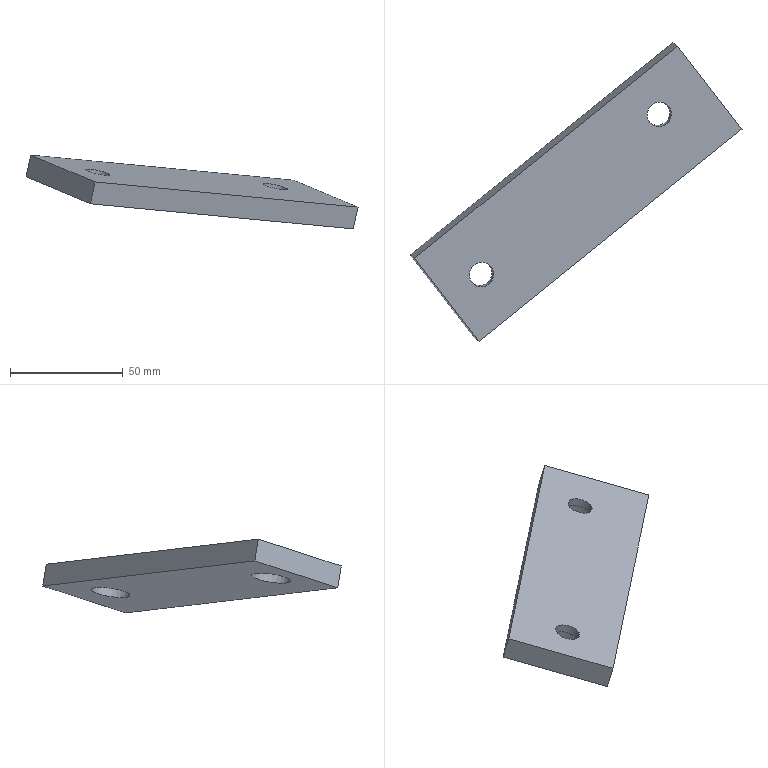Part | NX | features solid 2 | 1 solid | 12 faces | box 147.054 x 132.14 x 32.685 mm | volume 68266 mm3 | plane 8 | cylinder 4 | commonest cylinder face diameters 11 x2 17.5 x2
STEP:
#1=CARTESIAN_POINT('',(-157.138,684.094,54.963));
#2=VERTEX_POINT('',#1);
#3=CARTESIAN_POINT('',(-185.638,720.838,66.865));
#4=VERTEX_POINT('',#3);
#5=CARTESIAN_POINT('',(-185.638,720.838,66.865));
#6=DIRECTION('',(-0.5937,0.7655,0.248));
#7=VECTOR('',#6,1000.);
#8=LINE('',#5,#7);
#9=EDGE_CURVE('',#2,#4,#8,.T.);
#10=ORIENTED_EDGE('',*,*,#9,.T.);
#11=CARTESIAN_POINT('',(-187.758,722.323,57.206));
#12=VERTEX_POINT('',#11);
#13=CARTESIAN_POINT('',(-187.758,722.323,57.206));
#14=DIRECTION('',(0.212,-0.1485,0.9659));
#15=VECTOR('',#14,1000.);
#16=LINE('',#13,#15);
#17=EDGE_CURVE('',#12,#4,#16,.T.);
#18=ORIENTED_EDGE('',*,*,#17,.F.);
#19=CARTESIAN_POINT('',(-159.259,685.579,45.303));
#20=VERTEX_POINT('',#19);
#21=CARTESIAN_POINT('',(-187.758,722.323,57.206));
#22=DIRECTION('',(-0.5937,0.7655,0.248));
#23=VECTOR('',#22,1000.);
#24=LINE('',#21,#23);
#25=EDGE_CURVE('',#20,#12,#24,.T.);
#26=ORIENTED_EDGE('',*,*,#25,.F.);
#27=CARTESIAN_POINT('',(-159.259,685.579,45.303));
#28=DIRECTION('',(0.212,-0.1485,0.9659));
#29=VECTOR('',#28,1000.);
#30=LINE('',#27,#29);
#31=EDGE_CURVE('',#20,#2,#30,.T.);
#32=ORIENTED_EDGE('',*,*,#31,.T.);
#33=EDGE_LOOP('',(#10,#18,#26,#32));
#34=FACE_BOUND('',#33,.T.);
#35=CARTESIAN_POINT('',(-187.758,722.323,57.206));
#36=DIRECTION('',(0.7762,0.6261,-0.07415));
#37=DIRECTION('',(-0.6278,0.7784,0.));
#38=AXIS2_PLACEMENT_3D('',#35,#36,#37);
#39=PLANE('',#38);
#40=ADVANCED_FACE('',(#34),#39,.F.);
#41=CARTESIAN_POINT('',(-40.704,778.006,43.839));
#42=VERTEX_POINT('',#41);
#43=CARTESIAN_POINT('',(-40.704,778.006,43.839));
#44=DIRECTION('',(-0.7762,-0.6261,0.07415));
#45=VECTOR('',#44,1000.);
#46=LINE('',#43,#45);
#47=EDGE_CURVE('',#42,#2,#46,.T.);
#48=ORIENTED_EDGE('',*,*,#47,.T.);
#49=ORIENTED_EDGE('',*,*,#31,.F.);
#50=CARTESIAN_POINT('',(-42.824,779.49,34.18));
#51=VERTEX_POINT('',#50);
#52=CARTESIAN_POINT('',(-42.824,779.49,34.18));
#53=DIRECTION('',(-0.7762,-0.6261,0.07415));
#54=VECTOR('',#53,1000.);
#55=LINE('',#52,#54);
#56=EDGE_CURVE('',#51,#20,#55,.T.);
#57=ORIENTED_EDGE('',*,*,#56,.F.);
#58=CARTESIAN_POINT('',(-42.824,779.49,34.18));
#59=DIRECTION('',(0.212,-0.1485,0.9659));
#60=VECTOR('',#59,1000.);
#61=LINE('',#58,#60);
#62=EDGE_CURVE('',#51,#42,#61,.T.);
#63=ORIENTED_EDGE('',*,*,#62,.T.);
#64=EDGE_LOOP('',(#48,#49,#57,#63));
#65=FACE_BOUND('',#64,.T.);
#66=CARTESIAN_POINT('',(-42.824,779.49,34.18));
#67=DIRECTION('',(-0.5937,0.7655,0.248));
#68=DIRECTION('',(-0.7902,-0.6129,0.));
#69=AXIS2_PLACEMENT_3D('',#66,#67,#68);
#70=PLANE('',#69);
#71=ADVANCED_FACE('',(#65),#70,.F.);
#72=CARTESIAN_POINT('',(-69.203,814.75,55.742));
#73=VERTEX_POINT('',#72);
#74=CARTESIAN_POINT('',(-69.203,814.75,55.742));
#75=DIRECTION('',(-0.5937,0.7655,0.248));
#76=VECTOR('',#75,1000.);
#77=LINE('',#74,#76);
#78=EDGE_CURVE('',#42,#73,#77,.T.);
#79=ORIENTED_EDGE('',*,*,#78,.F.);
#80=ORIENTED_EDGE('',*,*,#62,.F.);
#81=CARTESIAN_POINT('',(-71.323,816.234,46.083));
#82=VERTEX_POINT('',#81);
#83=CARTESIAN_POINT('',(-71.323,816.234,46.083));
#84=DIRECTION('',(-0.5937,0.7655,0.248));
#85=VECTOR('',#84,1000.);
#86=LINE('',#83,#85);
#87=EDGE_CURVE('',#51,#82,#86,.T.);
#88=ORIENTED_EDGE('',*,*,#87,.T.);
#89=CARTESIAN_POINT('',(-71.323,816.234,46.083));
#90=DIRECTION('',(0.212,-0.1485,0.9659));
#91=VECTOR('',#90,1000.);
#92=LINE('',#89,#91);
#93=EDGE_CURVE('',#82,#73,#92,.T.);
#94=ORIENTED_EDGE('',*,*,#93,.T.);
#95=EDGE_LOOP('',(#79,#80,#88,#94));
#96=FACE_BOUND('',#95,.T.);
#97=CARTESIAN_POINT('',(-71.323,816.234,46.083));
#98=DIRECTION('',(0.7762,0.6261,-0.07415));
#99=DIRECTION('',(-0.6278,0.7784,0.));
#100=AXIS2_PLACEMENT_3D('',#97,#98,#99);
#101=PLANE('',#100);
#102=ADVANCED_FACE('',(#96),#101,.T.);
#103=CARTESIAN_POINT('',(-69.203,814.75,55.742));
#104=DIRECTION('',(-0.7762,-0.6261,0.07415));
#105=VECTOR('',#104,1000.);
#106=LINE('',#103,#105);
#107=EDGE_CURVE('',#73,#4,#106,.T.);
#108=ORIENTED_EDGE('',*,*,#107,.F.);
#109=ORIENTED_EDGE('',*,*,#93,.F.);
#110=CARTESIAN_POINT('',(-71.323,816.234,46.083));
#111=DIRECTION('',(-0.7762,-0.6261,0.07415));
#112=VECTOR('',#111,1000.);
#113=LINE('',#110,#112);
#114=EDGE_CURVE('',#82,#12,#113,.T.);
#115=ORIENTED_EDGE('',*,*,#114,.T.);
#116=ORIENTED_EDGE('',*,*,#17,.T.);
#117=EDGE_LOOP('',(#108,#109,#115,#116));
#118=FACE_BOUND('',#117,.T.);
#119=CARTESIAN_POINT('',(-71.323,816.234,46.083));
#120=DIRECTION('',(-0.5937,0.7655,0.248));
#121=DIRECTION('',(-0.7902,-0.6129,0.));
#122=AXIS2_PLACEMENT_3D('',#119,#120,#121);
#123=PLANE('',#122);
#124=ADVANCED_FACE('',(#118),#123,.T.);
#125=CARTESIAN_POINT('',(-149.62,715.081,47.722));
#126=VERTEX_POINT('',#125);
#127=CARTESIAN_POINT('',(-158.166,715.081,49.598));
#128=DIRECTION('',(0.212,-0.1485,0.9659));
#129=DIRECTION('',(0.9767,0.,-0.2144));
#130=AXIS2_PLACEMENT_3D('',#127,#128,#129);
#131=CIRCLE('',#130,8.75);
#132=EDGE_CURVE('',#126,#126,#131,.T.);
#133=ORIENTED_EDGE('',*,*,#132,.T.);
#134=EDGE_LOOP('',(#133));
#135=FACE_BOUND('',#134,.T.);
#136=CARTESIAN_POINT('',(-70.902,786.038,41.349));
#137=VERTEX_POINT('',#136);
#138=CARTESIAN_POINT('',(-79.448,786.038,43.225));
#139=DIRECTION('',(0.212,-0.1485,0.9659));
#140=DIRECTION('',(0.9767,0.,-0.2144));
#141=AXIS2_PLACEMENT_3D('',#138,#139,#140);
#142=CIRCLE('',#141,8.75);
#143=EDGE_CURVE('',#137,#137,#142,.T.);
#144=ORIENTED_EDGE('',*,*,#143,.T.);
#145=EDGE_LOOP('',(#144));
#146=FACE_BOUND('',#145,.T.);
#147=ORIENTED_EDGE('',*,*,#25,.T.);
#148=ORIENTED_EDGE('',*,*,#114,.F.);
#149=ORIENTED_EDGE('',*,*,#87,.F.);
#150=ORIENTED_EDGE('',*,*,#56,.T.);
#151=EDGE_LOOP('',(#147,#148,#149,#150));
#152=FACE_BOUND('',#151,.T.);
#153=CARTESIAN_POINT('',(-71.323,816.234,46.083));
#154=DIRECTION('',(0.212,-0.1485,0.9659));
#155=DIRECTION('',(-0.7762,-0.6261,0.07415));
#156=AXIS2_PLACEMENT_3D('',#153,#154,#155);
#157=PLANE('',#156);
#158=ADVANCED_FACE('',(#135,#146,#152),#157,.F.);
#159=CARTESIAN_POINT('',(-150.674,713.596,58.078));
#160=VERTEX_POINT('',#159);
#161=CARTESIAN_POINT('',(-156.046,713.596,59.257));
#162=DIRECTION('',(0.212,-0.1485,0.9659));
#163=DIRECTION('',(0.9767,0.,-0.2144));
#164=AXIS2_PLACEMENT_3D('',#161,#162,#163);
#165=CIRCLE('',#164,5.5);
#166=EDGE_CURVE('',#160,#160,#165,.T.);
#167=ORIENTED_EDGE('',*,*,#166,.F.);
#168=EDGE_LOOP('',(#167));
#169=FACE_BOUND('',#168,.T.);
#170=CARTESIAN_POINT('',(-71.956,784.553,51.705));
#171=VERTEX_POINT('',#170);
#172=CARTESIAN_POINT('',(-77.328,784.553,52.884));
#173=DIRECTION('',(0.212,-0.1485,0.9659));
#174=DIRECTION('',(0.9767,0.,-0.2144));
#175=AXIS2_PLACEMENT_3D('',#172,#173,#174);
#176=CIRCLE('',#175,5.5);
#177=EDGE_CURVE('',#171,#171,#176,.T.);
#178=ORIENTED_EDGE('',*,*,#177,.F.);
#179=EDGE_LOOP('',(#178));
#180=FACE_BOUND('',#179,.T.);
#181=ORIENTED_EDGE('',*,*,#9,.F.);
#182=ORIENTED_EDGE('',*,*,#47,.F.);
#183=ORIENTED_EDGE('',*,*,#78,.T.);
#184=ORIENTED_EDGE('',*,*,#107,.T.);
#185=EDGE_LOOP('',(#181,#182,#183,#184));
#186=FACE_BOUND('',#185,.T.);
#187=CARTESIAN_POINT('',(-69.203,814.75,55.742));
#188=DIRECTION('',(0.212,-0.1485,0.9659));
#189=DIRECTION('',(-0.7762,-0.6261,0.07415));
#190=AXIS2_PLACEMENT_3D('',#187,#188,#189);
#191=PLANE('',#190);
#192=ADVANCED_FACE('',(#169,#180,#186),#191,.T.);
#193=ORIENTED_EDGE('',*,*,#177,.T.);
#194=EDGE_LOOP('',(#193));
#195=FACE_BOUND('',#194,.T.);
#196=CARTESIAN_POINT('',(-72.74,785.103,48.131));
#197=VERTEX_POINT('',#196);
#198=CARTESIAN_POINT('',(-78.112,785.103,49.31));
#199=DIRECTION('',(0.212,-0.1485,0.9659));
#200=DIRECTION('',(0.9767,0.,-0.2144));
#201=AXIS2_PLACEMENT_3D('',#198,#199,#200);
#202=CIRCLE('',#201,5.5);
#203=EDGE_CURVE('',#197,#197,#202,.T.);
#204=ORIENTED_EDGE('',*,*,#203,.F.);
#205=EDGE_LOOP('',(#204));
#206=FACE_BOUND('',#205,.T.);
#207=CARTESIAN_POINT('',(-68.848,778.615,91.521));
#208=DIRECTION('',(0.212,-0.1485,0.9659));
#209=DIRECTION('',(0.9767,0.,-0.2144));
#210=AXIS2_PLACEMENT_3D('',#207,#208,#209);
#211=CYLINDRICAL_SURFACE('',#210,5.5);
#212=ADVANCED_FACE('',(#195,#206),#211,.F.);
#213=ORIENTED_EDGE('',*,*,#203,.T.);
#214=EDGE_LOOP('',(#213));
#215=FACE_BOUND('',#214,.T.);
#216=CARTESIAN_POINT('',(-69.566,785.103,47.435));
#217=VERTEX_POINT('',#216);
#218=CARTESIAN_POINT('',(-78.112,785.103,49.31));
#219=DIRECTION('',(0.212,-0.1485,0.9659));
#220=DIRECTION('',(0.9767,0.,-0.2144));
#221=AXIS2_PLACEMENT_3D('',#218,#219,#220);
#222=CIRCLE('',#221,8.75);
#223=EDGE_CURVE('',#217,#217,#222,.T.);
#224=ORIENTED_EDGE('',*,*,#223,.F.);
#225=EDGE_LOOP('',(#224));
#226=FACE_BOUND('',#225,.T.);
#227=CARTESIAN_POINT('',(-78.112,785.103,49.31));
#228=DIRECTION('',(0.212,-0.1485,0.9659));
#229=DIRECTION('',(0.9767,0.,-0.2144));
#230=AXIS2_PLACEMENT_3D('',#227,#228,#229);
#231=PLANE('',#230);
#232=ADVANCED_FACE('',(#215,#226),#231,.F.);
#233=ORIENTED_EDGE('',*,*,#223,.T.);
#234=EDGE_LOOP('',(#233));
#235=FACE_BOUND('',#234,.T.);
#236=ORIENTED_EDGE('',*,*,#143,.F.);
#237=EDGE_LOOP('',(#236));
#238=FACE_BOUND('',#237,.T.);
#239=CARTESIAN_POINT('',(-79.448,786.038,43.225));
#240=DIRECTION('',(0.212,-0.1485,0.9659));
#241=DIRECTION('',(0.9767,0.,-0.2144));
#242=AXIS2_PLACEMENT_3D('',#239,#240,#241);
#243=CYLINDRICAL_SURFACE('',#242,8.75);
#244=ADVANCED_FACE('',(#235,#238),#243,.F.);
#245=ORIENTED_EDGE('',*,*,#166,.T.);
#246=EDGE_LOOP('',(#245));
#247=FACE_BOUND('',#246,.T.);
#248=CARTESIAN_POINT('',(-151.458,714.146,54.504));
#249=VERTEX_POINT('',#248);
#250=CARTESIAN_POINT('',(-156.83,714.146,55.683));
#251=DIRECTION('',(0.212,-0.1485,0.9659));
#252=DIRECTION('',(0.9767,0.,-0.2144));
#253=AXIS2_PLACEMENT_3D('',#250,#251,#252);
#254=CIRCLE('',#253,5.5);
#255=EDGE_CURVE('',#249,#249,#254,.T.);
#256=ORIENTED_EDGE('',*,*,#255,.F.);
#257=EDGE_LOOP('',(#256));
#258=FACE_BOUND('',#257,.T.);
#259=CARTESIAN_POINT('',(-147.565,707.658,97.894));
#260=DIRECTION('',(0.212,-0.1485,0.9659));
#261=DIRECTION('',(0.9767,0.,-0.2144));
#262=AXIS2_PLACEMENT_3D('',#259,#260,#261);
#263=CYLINDRICAL_SURFACE('',#262,5.5);
#264=ADVANCED_FACE('',(#247,#258),#263,.F.);
#265=ORIENTED_EDGE('',*,*,#255,.T.);
#266=EDGE_LOOP('',(#265));
#267=FACE_BOUND('',#266,.T.);
#268=CARTESIAN_POINT('',(-148.284,714.146,53.807));
#269=VERTEX_POINT('',#268);
#270=CARTESIAN_POINT('',(-156.83,714.146,55.683));
#271=DIRECTION('',(0.212,-0.1485,0.9659));
#272=DIRECTION('',(0.9767,0.,-0.2144));
#273=AXIS2_PLACEMENT_3D('',#270,#271,#272);
#274=CIRCLE('',#273,8.75);
#275=EDGE_CURVE('',#269,#269,#274,.T.);
#276=ORIENTED_EDGE('',*,*,#275,.F.);
#277=EDGE_LOOP('',(#276));
#278=FACE_BOUND('',#277,.T.);
#279=CARTESIAN_POINT('',(-156.83,714.146,55.683));
#280=DIRECTION('',(0.212,-0.1485,0.9659));
#281=DIRECTION('',(0.9767,0.,-0.2144));
#282=AXIS2_PLACEMENT_3D('',#279,#280,#281);
#283=PLANE('',#282);
#284=ADVANCED_FACE('',(#267,#278),#283,.F.);
#285=ORIENTED_EDGE('',*,*,#275,.T.);
#286=EDGE_LOOP('',(#285));
#287=FACE_BOUND('',#286,.T.);
#288=ORIENTED_EDGE('',*,*,#132,.F.);
#289=EDGE_LOOP('',(#288));
#290=FACE_BOUND('',#289,.T.);
#291=CARTESIAN_POINT('',(-158.166,715.081,49.598));
#292=DIRECTION('',(0.212,-0.1485,0.9659));
#293=DIRECTION('',(0.9767,0.,-0.2144));
#294=AXIS2_PLACEMENT_3D('',#291,#292,#293);
#295=CYLINDRICAL_SURFACE('',#294,8.75);
#296=ADVANCED_FACE('',(#287,#290),#295,.F.);
#297=CLOSED_SHELL('',(#40,#71,#102,#124,#158,#192,#212,#232,#244,#264,#284,#296));
#298=MANIFOLD_SOLID_BREP('',#297);
#299=(LENGTH_UNIT()NAMED_UNIT(*)SI_UNIT(.MILLI.,.METRE.));
#300=UNCERTAINTY_MEASURE_WITH_UNIT(LENGTH_MEASURE(0.00001),#299,'','');
#301=(NAMED_UNIT(*)PLANE_ANGLE_UNIT()SI_UNIT($,.RADIAN.));
#302=(NAMED_UNIT(*)SI_UNIT($,.STERADIAN.)SOLID_ANGLE_UNIT());
#303=(GEOMETRIC_REPRESENTATION_CONTEXT(3)GLOBAL_UNCERTAINTY_ASSIGNED_CONTEXT((#300))GLOBAL_UNIT_ASSIGNED_CONTEXT((#299,#301,#302))REPRESENTATION_CONTEXT('',''));
#304=ADVANCED_BREP_SHAPE_REPRESENTATION('',(#298),#303);